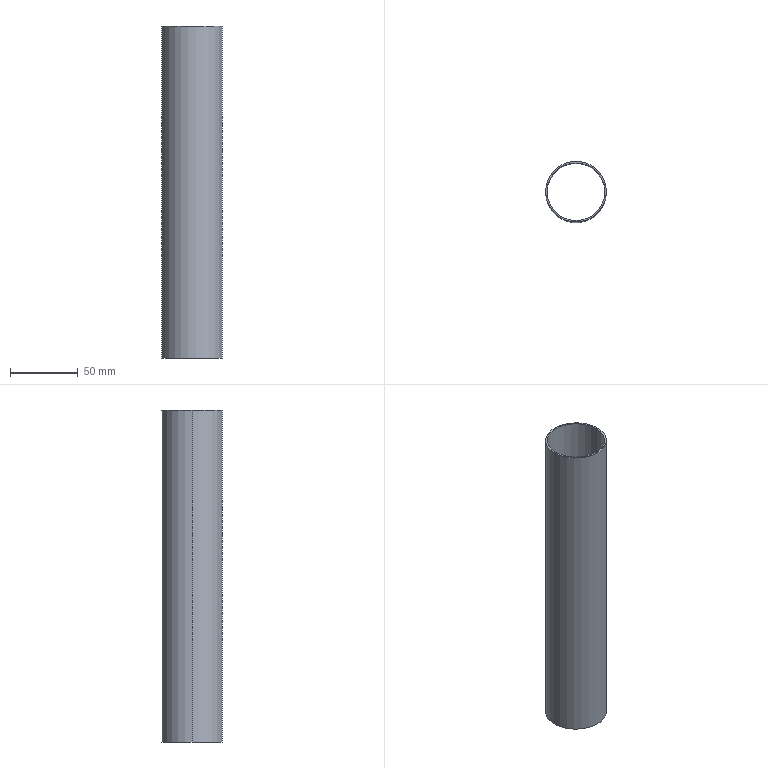Part | SolidWorks | features Extrusion 1 | 1 solid | 6 faces | box 45 x 45 x 245 mm | volume 40455 mm3 | cylinder 4 | plane 2 | commonest cylinder face diameters 42.6 x2 45 x2
STEP:
#1=CARTESIAN_POINT('',(-21.3,0.,245.));
#2=VERTEX_POINT('',#1);
#3=CARTESIAN_POINT('',(21.3,0.,245.));
#4=VERTEX_POINT('',#3);
#5=CARTESIAN_POINT('',(0.,0.,245.));
#6=DIRECTION('',(0.,0.,1.));
#7=DIRECTION('',(1.,0.,0.));
#8=AXIS2_PLACEMENT_3D('',#5,#6,#7);
#9=CIRCLE('',#8,21.3);
#10=EDGE_CURVE('',#2,#4,#9,.T.);
#11=ORIENTED_EDGE('',*,*,#10,.T.);
#12=CARTESIAN_POINT('',(21.3,0.,0.));
#13=VERTEX_POINT('',#12);
#14=CARTESIAN_POINT('',(21.3,0.,245.));
#15=DIRECTION('',(0.,0.,-1.));
#16=VECTOR('',#15,1000.);
#17=LINE('',#14,#16);
#18=EDGE_CURVE('',#4,#13,#17,.T.);
#19=ORIENTED_EDGE('',*,*,#18,.T.);
#20=CARTESIAN_POINT('',(-21.3,0.,0.));
#21=VERTEX_POINT('',#20);
#22=CARTESIAN_POINT('',(0.,0.,0.));
#23=DIRECTION('',(0.,0.,1.));
#24=DIRECTION('',(1.,0.,0.));
#25=AXIS2_PLACEMENT_3D('',#22,#23,#24);
#26=CIRCLE('',#25,21.3);
#27=EDGE_CURVE('',#21,#13,#26,.T.);
#28=ORIENTED_EDGE('',*,*,#27,.F.);
#29=CARTESIAN_POINT('',(-21.3,0.,245.));
#30=DIRECTION('',(0.,0.,-1.));
#31=VECTOR('',#30,1000.);
#32=LINE('',#29,#31);
#33=EDGE_CURVE('',#2,#21,#32,.T.);
#34=ORIENTED_EDGE('',*,*,#33,.F.);
#35=EDGE_LOOP('',(#11,#19,#28,#34));
#36=FACE_OUTER_BOUND('',#35,.T.);
#37=CARTESIAN_POINT('',(0.,0.,245.));
#38=DIRECTION('',(0.,0.,-1.));
#39=DIRECTION('',(-1.,0.,0.));
#40=AXIS2_PLACEMENT_3D('',#37,#38,#39);
#41=CYLINDRICAL_SURFACE('',#40,21.3);
#42=ADVANCED_FACE('',(#36),#41,.F.);
#43=CARTESIAN_POINT('',(22.5,0.,245.));
#44=VERTEX_POINT('',#43);
#45=CARTESIAN_POINT('',(-22.5,0.,245.));
#46=VERTEX_POINT('',#45);
#47=CARTESIAN_POINT('',(0.,0.,245.));
#48=DIRECTION('',(0.,0.,1.));
#49=DIRECTION('',(1.,0.,0.));
#50=AXIS2_PLACEMENT_3D('',#47,#48,#49);
#51=CIRCLE('',#50,22.5);
#52=EDGE_CURVE('',#44,#46,#51,.T.);
#53=ORIENTED_EDGE('',*,*,#52,.F.);
#54=CARTESIAN_POINT('',(22.5,0.,0.));
#55=VERTEX_POINT('',#54);
#56=CARTESIAN_POINT('',(22.5,0.,245.));
#57=DIRECTION('',(0.,0.,-1.));
#58=VECTOR('',#57,1000.);
#59=LINE('',#56,#58);
#60=EDGE_CURVE('',#44,#55,#59,.T.);
#61=ORIENTED_EDGE('',*,*,#60,.T.);
#62=CARTESIAN_POINT('',(-22.5,0.,0.));
#63=VERTEX_POINT('',#62);
#64=CARTESIAN_POINT('',(0.,0.,0.));
#65=DIRECTION('',(0.,0.,1.));
#66=DIRECTION('',(1.,0.,0.));
#67=AXIS2_PLACEMENT_3D('',#64,#65,#66);
#68=CIRCLE('',#67,22.5);
#69=EDGE_CURVE('',#55,#63,#68,.T.);
#70=ORIENTED_EDGE('',*,*,#69,.T.);
#71=CARTESIAN_POINT('',(-22.5,0.,245.));
#72=DIRECTION('',(0.,0.,-1.));
#73=VECTOR('',#72,1000.);
#74=LINE('',#71,#73);
#75=EDGE_CURVE('',#46,#63,#74,.T.);
#76=ORIENTED_EDGE('',*,*,#75,.F.);
#77=EDGE_LOOP('',(#53,#61,#70,#76));
#78=FACE_OUTER_BOUND('',#77,.T.);
#79=CARTESIAN_POINT('',(0.,0.,245.));
#80=DIRECTION('',(0.,0.,-1.));
#81=DIRECTION('',(-1.,0.,0.));
#82=AXIS2_PLACEMENT_3D('',#79,#80,#81);
#83=CYLINDRICAL_SURFACE('',#82,22.5);
#84=ADVANCED_FACE('',(#78),#83,.T.);
#85=CARTESIAN_POINT('',(0.,0.,245.));
#86=DIRECTION('',(0.,0.,1.));
#87=DIRECTION('',(1.,0.,0.));
#88=AXIS2_PLACEMENT_3D('',#85,#86,#87);
#89=CIRCLE('',#88,22.5);
#90=EDGE_CURVE('',#46,#44,#89,.T.);
#91=ORIENTED_EDGE('',*,*,#90,.T.);
#92=ORIENTED_EDGE('',*,*,#52,.T.);
#93=EDGE_LOOP('',(#91,#92));
#94=FACE_OUTER_BOUND('',#93,.T.);
#95=ORIENTED_EDGE('',*,*,#10,.F.);
#96=CARTESIAN_POINT('',(0.,0.,245.));
#97=DIRECTION('',(0.,0.,1.));
#98=DIRECTION('',(1.,0.,0.));
#99=AXIS2_PLACEMENT_3D('',#96,#97,#98);
#100=CIRCLE('',#99,21.3);
#101=EDGE_CURVE('',#4,#2,#100,.T.);
#102=ORIENTED_EDGE('',*,*,#101,.F.);
#103=EDGE_LOOP('',(#95,#102));
#104=FACE_BOUND('',#103,.T.);
#105=CARTESIAN_POINT('',(0.,0.,245.));
#106=DIRECTION('',(0.,0.,1.));
#107=DIRECTION('',(1.,0.,0.));
#108=AXIS2_PLACEMENT_3D('',#105,#106,#107);
#109=PLANE('',#108);
#110=ADVANCED_FACE('',(#94,#104),#109,.T.);
#111=CARTESIAN_POINT('',(0.,0.,0.));
#112=DIRECTION('',(0.,0.,1.));
#113=DIRECTION('',(1.,0.,0.));
#114=AXIS2_PLACEMENT_3D('',#111,#112,#113);
#115=CIRCLE('',#114,22.5);
#116=EDGE_CURVE('',#63,#55,#115,.T.);
#117=ORIENTED_EDGE('',*,*,#116,.F.);
#118=ORIENTED_EDGE('',*,*,#69,.F.);
#119=EDGE_LOOP('',(#117,#118));
#120=FACE_OUTER_BOUND('',#119,.T.);
#121=ORIENTED_EDGE('',*,*,#27,.T.);
#122=CARTESIAN_POINT('',(0.,0.,0.));
#123=DIRECTION('',(0.,0.,1.));
#124=DIRECTION('',(1.,0.,0.));
#125=AXIS2_PLACEMENT_3D('',#122,#123,#124);
#126=CIRCLE('',#125,21.3);
#127=EDGE_CURVE('',#13,#21,#126,.T.);
#128=ORIENTED_EDGE('',*,*,#127,.T.);
#129=EDGE_LOOP('',(#121,#128));
#130=FACE_BOUND('',#129,.T.);
#131=CARTESIAN_POINT('',(0.,0.,0.));
#132=DIRECTION('',(0.,0.,1.));
#133=DIRECTION('',(1.,0.,0.));
#134=AXIS2_PLACEMENT_3D('',#131,#132,#133);
#135=PLANE('',#134);
#136=ADVANCED_FACE('',(#120,#130),#135,.F.);
#137=ORIENTED_EDGE('',*,*,#60,.F.);
#138=ORIENTED_EDGE('',*,*,#90,.F.);
#139=ORIENTED_EDGE('',*,*,#75,.T.);
#140=ORIENTED_EDGE('',*,*,#116,.T.);
#141=EDGE_LOOP('',(#137,#138,#139,#140));
#142=FACE_OUTER_BOUND('',#141,.T.);
#143=CARTESIAN_POINT('',(0.,0.,245.));
#144=DIRECTION('',(0.,0.,-1.));
#145=DIRECTION('',(-1.,0.,0.));
#146=AXIS2_PLACEMENT_3D('',#143,#144,#145);
#147=CYLINDRICAL_SURFACE('',#146,22.5);
#148=ADVANCED_FACE('',(#142),#147,.T.);
#149=ORIENTED_EDGE('',*,*,#18,.F.);
#150=ORIENTED_EDGE('',*,*,#101,.T.);
#151=ORIENTED_EDGE('',*,*,#33,.T.);
#152=ORIENTED_EDGE('',*,*,#127,.F.);
#153=EDGE_LOOP('',(#149,#150,#151,#152));
#154=FACE_OUTER_BOUND('',#153,.T.);
#155=CARTESIAN_POINT('',(0.,0.,245.));
#156=DIRECTION('',(0.,0.,-1.));
#157=DIRECTION('',(-1.,0.,0.));
#158=AXIS2_PLACEMENT_3D('',#155,#156,#157);
#159=CYLINDRICAL_SURFACE('',#158,21.3);
#160=ADVANCED_FACE('',(#154),#159,.F.);
#161=CLOSED_SHELL('',(#42,#84,#110,#136,#148,#160));
#162=MANIFOLD_SOLID_BREP('',#161);
#163=CARTESIAN_POINT('',(0.,0.,0.));
#164=DIRECTION('',(0.,0.,1.));
#165=DIRECTION('',(1.,0.,0.));
#166=AXIS2_PLACEMENT_3D('',#163,#164,#165);
#167=(LENGTH_UNIT()NAMED_UNIT(*)SI_UNIT(.MILLI.,.METRE.));
#168=UNCERTAINTY_MEASURE_WITH_UNIT(LENGTH_MEASURE(0.00001),#167,'','');
#169=(NAMED_UNIT(*)PLANE_ANGLE_UNIT()SI_UNIT($,.RADIAN.));
#170=(NAMED_UNIT(*)SI_UNIT($,.STERADIAN.)SOLID_ANGLE_UNIT());
#171=(GEOMETRIC_REPRESENTATION_CONTEXT(3)GLOBAL_UNCERTAINTY_ASSIGNED_CONTEXT((#168))GLOBAL_UNIT_ASSIGNED_CONTEXT((#167,#169,#170))REPRESENTATION_CONTEXT('',''));
#172=ADVANCED_BREP_SHAPE_REPRESENTATION('',(#162,#166),#171);